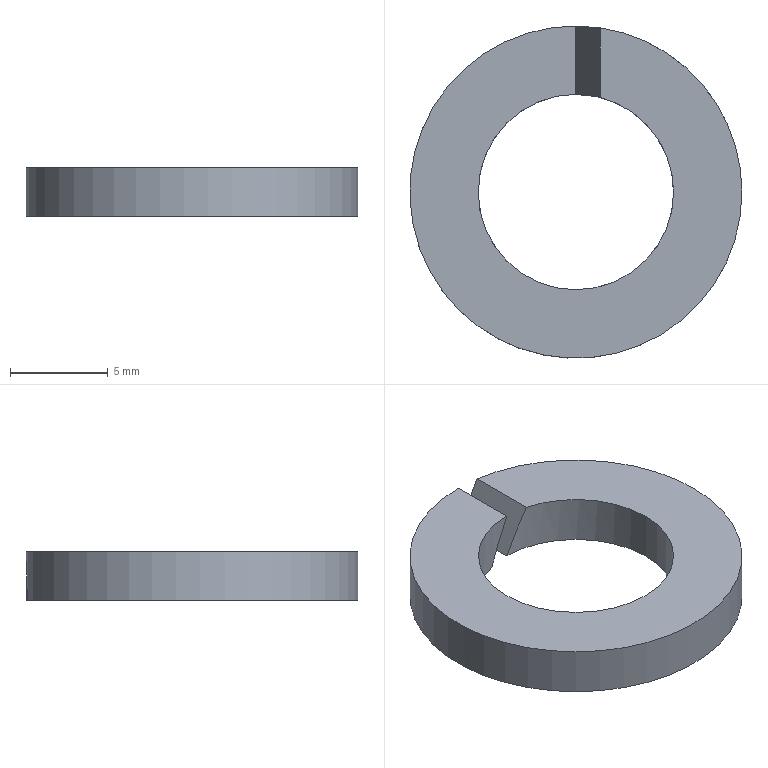Part | STEP file | D10_GB9074_26 | 1 solid | 8 faces | box 17 x 17 x 2.5 mm | volume 360.129 mm3 | plane 4 | cylinder 4 | commonest cylinder face diameters 10 x2 17 x2
STEP:
#1=CARTESIAN_POINT('',(0.,0.,0.));
#2=DIRECTION('',(0.,0.,1.));
#3=DIRECTION('',(1.,0.,0.));
#4=AXIS2_PLACEMENT_3D('',#1,#2,#3);
#5=CARTESIAN_POINT('',(-1.25,4.841,0.));
#6=VERTEX_POINT('',#5);
#7=CARTESIAN_POINT('',(-1.25,8.408,0.));
#8=VERTEX_POINT('',#7);
#9=CARTESIAN_POINT('',(-1.25,4.841,0.));
#10=DIRECTION('',(0.,1.,0.));
#11=VECTOR('',#10,1.);
#12=LINE('',#9,#11);
#13=CARTESIAN_POINT('',(0.,0.,0.));
#14=DIRECTION('',(0.,0.,1.));
#15=DIRECTION('',(1.,0.,0.));
#16=AXIS2_PLACEMENT_3D('',#13,#14,#15);
#17=PLANE('',#16);
#18=CARTESIAN_POINT('',(-1.25,4.841));
#19=DIRECTION('',(0.,1.));
#20=VECTOR('',#19,1.);
#21=LINE('',#18,#20);
#22=(GEOMETRIC_REPRESENTATION_CONTEXT(2)PARAMETRIC_REPRESENTATION_CONTEXT()REPRESENTATION_CONTEXT('',''));
#23=DEFINITIONAL_REPRESENTATION('',(#21),#22);
#24=PCURVE('',#17,#23);
#25=CARTESIAN_POINT('',(-1.25,0.,0.));
#26=DIRECTION('',(-0.8944,0.,0.4472));
#27=DIRECTION('',(0.4472,0.,0.8944));
#28=AXIS2_PLACEMENT_3D('',#25,#26,#27);
#29=PLANE('',#28);
#30=CARTESIAN_POINT('',(0.,4.841));
#31=DIRECTION('',(0.,1.));
#32=VECTOR('',#31,1.);
#33=LINE('',#30,#32);
#34=(GEOMETRIC_REPRESENTATION_CONTEXT(2)PARAMETRIC_REPRESENTATION_CONTEXT()REPRESENTATION_CONTEXT('',''));
#35=DEFINITIONAL_REPRESENTATION('',(#33),#34);
#36=PCURVE('',#29,#35);
#37=SURFACE_CURVE('',#12,(#24,#36),.PCURVE_S1.);
#38=EDGE_CURVE('',#6,#8,#37,.T.);
#39=ORIENTED_EDGE('',*,*,#38,.T.);
#40=CARTESIAN_POINT('',(8.5,0.,0.));
#41=VERTEX_POINT('',#40);
#42=CARTESIAN_POINT('',(0.,0.,0.));
#43=DIRECTION('',(0.,0.,-1.));
#44=DIRECTION('',(1.,0.,0.));
#45=AXIS2_PLACEMENT_3D('',#42,#43,#44);
#46=CIRCLE('',#45,8.5);
#47=CARTESIAN_POINT('',(8.5,0.));
#48=CARTESIAN_POINT('',(8.5,-14.722));
#49=CARTESIAN_POINT('',(-4.25,-7.361));
#50=CARTESIAN_POINT('',(-17.,0.));
#51=CARTESIAN_POINT('',(-4.25,7.361));
#52=CARTESIAN_POINT('',(8.5,14.722));
#53=CARTESIAN_POINT('',(8.5,0.));
#54=(BOUNDED_CURVE()B_SPLINE_CURVE(2,(#47,#48,#49,#50,#51,#52,#53),.UNSPECIFIED.,.T.,.F.)B_SPLINE_CURVE_WITH_KNOTS((1,2,2,2,2,1),(-2.094,0.,2.094,4.189,6.283,8.378),.UNSPECIFIED.)CURVE()GEOMETRIC_REPRESENTATION_ITEM()RATIONAL_B_SPLINE_CURVE((1.,0.5,1.,0.5,1.,0.5,1.))REPRESENTATION_ITEM(''));
#55=(GEOMETRIC_REPRESENTATION_CONTEXT(2)PARAMETRIC_REPRESENTATION_CONTEXT()REPRESENTATION_CONTEXT('',''));
#56=DEFINITIONAL_REPRESENTATION('',(#54),#55);
#57=PCURVE('',#17,#56);
#58=CARTESIAN_POINT('',(0.,0.,0.));
#59=DIRECTION('',(0.,0.,1.));
#60=DIRECTION('',(1.,0.,0.));
#61=AXIS2_PLACEMENT_3D('',#58,#59,#60);
#62=CYLINDRICAL_SURFACE('',#61,8.5);
#63=CARTESIAN_POINT('',(6.283,0.));
#64=DIRECTION('',(-1.,0.));
#65=VECTOR('',#64,1.);
#66=LINE('',#63,#65);
#67=(GEOMETRIC_REPRESENTATION_CONTEXT(2)PARAMETRIC_REPRESENTATION_CONTEXT()REPRESENTATION_CONTEXT('',''));
#68=DEFINITIONAL_REPRESENTATION('',(#66),#67);
#69=PCURVE('',#62,#68);
#70=SURFACE_CURVE('',#46,(#57,#69),.PCURVE_S1.);
#71=EDGE_CURVE('',#41,#8,#70,.T.);
#72=ORIENTED_EDGE('',*,*,#71,.F.);
#73=CARTESIAN_POINT('',(0.,8.5,0.));
#74=VERTEX_POINT('',#73);
#75=CARTESIAN_POINT('',(0.,0.,0.));
#76=DIRECTION('',(0.,0.,1.));
#77=DIRECTION('',(1.,0.,0.));
#78=AXIS2_PLACEMENT_3D('',#75,#76,#77);
#79=CIRCLE('',#78,8.5);
#80=CARTESIAN_POINT('',(0.,0.));
#81=DIRECTION('',(1.,0.));
#82=AXIS2_PLACEMENT_2D('',#80,#81);
#83=CIRCLE('',#82,8.5);
#84=(GEOMETRIC_REPRESENTATION_CONTEXT(2)PARAMETRIC_REPRESENTATION_CONTEXT()REPRESENTATION_CONTEXT('',''));
#85=DEFINITIONAL_REPRESENTATION('',(#83),#84);
#86=PCURVE('',#17,#85);
#87=CARTESIAN_POINT('',(0.,0.,0.));
#88=DIRECTION('',(0.,0.,1.));
#89=DIRECTION('',(1.,0.,0.));
#90=AXIS2_PLACEMENT_3D('',#87,#88,#89);
#91=CYLINDRICAL_SURFACE('',#90,8.5);
#92=CARTESIAN_POINT('',(0.,0.));
#93=DIRECTION('',(1.,0.));
#94=VECTOR('',#93,1.);
#95=LINE('',#92,#94);
#96=(GEOMETRIC_REPRESENTATION_CONTEXT(2)PARAMETRIC_REPRESENTATION_CONTEXT()REPRESENTATION_CONTEXT('',''));
#97=DEFINITIONAL_REPRESENTATION('',(#95),#96);
#98=PCURVE('',#91,#97);
#99=SURFACE_CURVE('',#79,(#86,#98),.PCURVE_S1.);
#100=EDGE_CURVE('',#41,#74,#99,.T.);
#101=ORIENTED_EDGE('',*,*,#100,.T.);
#102=CARTESIAN_POINT('',(0.,5.,0.));
#103=VERTEX_POINT('',#102);
#104=CARTESIAN_POINT('',(0.,5.,0.));
#105=DIRECTION('',(0.,1.,0.));
#106=VECTOR('',#105,1.);
#107=LINE('',#104,#106);
#108=CARTESIAN_POINT('',(0.,5.));
#109=DIRECTION('',(0.,1.));
#110=VECTOR('',#109,1.);
#111=LINE('',#108,#110);
#112=(GEOMETRIC_REPRESENTATION_CONTEXT(2)PARAMETRIC_REPRESENTATION_CONTEXT()REPRESENTATION_CONTEXT('',''));
#113=DEFINITIONAL_REPRESENTATION('',(#111),#112);
#114=PCURVE('',#17,#113);
#115=CARTESIAN_POINT('',(1.25,0.,2.5));
#116=DIRECTION('',(0.8944,0.,-0.4472));
#117=DIRECTION('',(-0.4472,0.,-0.8944));
#118=AXIS2_PLACEMENT_3D('',#115,#116,#117);
#119=PLANE('',#118);
#120=CARTESIAN_POINT('',(2.795,5.));
#121=DIRECTION('',(0.,1.));
#122=VECTOR('',#121,1.);
#123=LINE('',#120,#122);
#124=(GEOMETRIC_REPRESENTATION_CONTEXT(2)PARAMETRIC_REPRESENTATION_CONTEXT()REPRESENTATION_CONTEXT('',''));
#125=DEFINITIONAL_REPRESENTATION('',(#123),#124);
#126=PCURVE('',#119,#125);
#127=SURFACE_CURVE('',#107,(#114,#126),.PCURVE_S1.);
#128=EDGE_CURVE('',#103,#74,#127,.T.);
#129=ORIENTED_EDGE('',*,*,#128,.F.);
#130=CARTESIAN_POINT('',(5.,0.,0.));
#131=VERTEX_POINT('',#130);
#132=CARTESIAN_POINT('',(0.,0.,0.));
#133=DIRECTION('',(0.,0.,-1.));
#134=DIRECTION('',(0.,1.,0.));
#135=AXIS2_PLACEMENT_3D('',#132,#133,#134);
#136=CIRCLE('',#135,5.);
#137=CARTESIAN_POINT('',(0.,5.));
#138=CARTESIAN_POINT('',(8.66,5.));
#139=CARTESIAN_POINT('',(4.33,-2.5));
#140=CARTESIAN_POINT('',(0.,-10.));
#141=CARTESIAN_POINT('',(-4.33,-2.5));
#142=CARTESIAN_POINT('',(-8.66,5.));
#143=CARTESIAN_POINT('',(0.,5.));
#144=(BOUNDED_CURVE()B_SPLINE_CURVE(2,(#137,#138,#139,#140,#141,#142,#143),.UNSPECIFIED.,.T.,.F.)B_SPLINE_CURVE_WITH_KNOTS((1,2,2,2,2,1),(-2.094,0.,2.094,4.189,6.283,8.378),.UNSPECIFIED.)CURVE()GEOMETRIC_REPRESENTATION_ITEM()RATIONAL_B_SPLINE_CURVE((1.,0.5,1.,0.5,1.,0.5,1.))REPRESENTATION_ITEM(''));
#145=(GEOMETRIC_REPRESENTATION_CONTEXT(2)PARAMETRIC_REPRESENTATION_CONTEXT()REPRESENTATION_CONTEXT('',''));
#146=DEFINITIONAL_REPRESENTATION('',(#144),#145);
#147=PCURVE('',#17,#146);
#148=CARTESIAN_POINT('',(0.,0.,0.));
#149=DIRECTION('',(0.,0.,1.));
#150=DIRECTION('',(1.,0.,0.));
#151=AXIS2_PLACEMENT_3D('',#148,#149,#150);
#152=CYLINDRICAL_SURFACE('',#151,5.);
#153=CARTESIAN_POINT('',(1.571,0.));
#154=DIRECTION('',(-1.,0.));
#155=VECTOR('',#154,1.);
#156=LINE('',#153,#155);
#157=(GEOMETRIC_REPRESENTATION_CONTEXT(2)PARAMETRIC_REPRESENTATION_CONTEXT()REPRESENTATION_CONTEXT('',''));
#158=DEFINITIONAL_REPRESENTATION('',(#156),#157);
#159=PCURVE('',#152,#158);
#160=SURFACE_CURVE('',#136,(#147,#159),.PCURVE_S1.);
#161=EDGE_CURVE('',#103,#131,#160,.T.);
#162=ORIENTED_EDGE('',*,*,#161,.T.);
#163=CARTESIAN_POINT('',(0.,0.,0.));
#164=DIRECTION('',(0.,0.,1.));
#165=DIRECTION('',(-0.25,0.9682,0.));
#166=AXIS2_PLACEMENT_3D('',#163,#164,#165);
#167=CIRCLE('',#166,5.);
#168=CARTESIAN_POINT('',(0.,0.));
#169=DIRECTION('',(-0.25,0.9682));
#170=AXIS2_PLACEMENT_2D('',#168,#169);
#171=CIRCLE('',#170,5.);
#172=(GEOMETRIC_REPRESENTATION_CONTEXT(2)PARAMETRIC_REPRESENTATION_CONTEXT()REPRESENTATION_CONTEXT('',''));
#173=DEFINITIONAL_REPRESENTATION('',(#171),#172);
#174=PCURVE('',#17,#173);
#175=CARTESIAN_POINT('',(0.,0.,0.));
#176=DIRECTION('',(0.,0.,1.));
#177=DIRECTION('',(1.,0.,0.));
#178=AXIS2_PLACEMENT_3D('',#175,#176,#177);
#179=CYLINDRICAL_SURFACE('',#178,5.);
#180=CARTESIAN_POINT('',(1.823,0.));
#181=DIRECTION('',(1.,0.));
#182=VECTOR('',#181,1.);
#183=LINE('',#180,#182);
#184=(GEOMETRIC_REPRESENTATION_CONTEXT(2)PARAMETRIC_REPRESENTATION_CONTEXT()REPRESENTATION_CONTEXT('',''));
#185=DEFINITIONAL_REPRESENTATION('',(#183),#184);
#186=PCURVE('',#179,#185);
#187=SURFACE_CURVE('',#167,(#174,#186),.PCURVE_S1.);
#188=EDGE_CURVE('',#6,#131,#187,.T.);
#189=ORIENTED_EDGE('',*,*,#188,.F.);
#190=EDGE_LOOP('',(#39,#72,#101,#129,#162,#189));
#191=FACE_BOUND('',#190,.F.);
#192=ADVANCED_FACE('',(#191),#17,.F.);
#193=CARTESIAN_POINT('',(0.,5.,2.5));
#194=VERTEX_POINT('',#193);
#195=CARTESIAN_POINT('',(0.,5.,2.5));
#196=CARTESIAN_POINT('',(-0.418,5.,1.664));
#197=CARTESIAN_POINT('',(-0.8347,4.948,0.8305));
#198=CARTESIAN_POINT('',(-1.25,4.841,0.));
#199=B_SPLINE_CURVE_WITH_KNOTS('',3,(#195,#196,#197,#198),.UNSPECIFIED.,.F.,.F.,(4,4),(0.,1.),.PIECEWISE_BEZIER_KNOTS.);
#200=CARTESIAN_POINT('',(2.795,5.));
#201=CARTESIAN_POINT('',(1.86,5.));
#202=CARTESIAN_POINT('',(0.9286,4.948));
#203=CARTESIAN_POINT('',(0.,4.841));
#204=B_SPLINE_CURVE_WITH_KNOTS('',3,(#200,#201,#202,#203),.UNSPECIFIED.,.F.,.F.,(4,4),(0.,1.),.PIECEWISE_BEZIER_KNOTS.);
#205=(GEOMETRIC_REPRESENTATION_CONTEXT(2)PARAMETRIC_REPRESENTATION_CONTEXT()REPRESENTATION_CONTEXT('',''));
#206=DEFINITIONAL_REPRESENTATION('',(#204),#205);
#207=PCURVE('',#29,#206);
#208=CARTESIAN_POINT('',(1.571,2.5));
#209=CARTESIAN_POINT('',(1.575,2.462));
#210=CARTESIAN_POINT('',(1.582,2.386));
#211=CARTESIAN_POINT('',(1.594,2.272));
#212=CARTESIAN_POINT('',(1.605,2.158));
#213=CARTESIAN_POINT('',(1.616,2.044));
#214=CARTESIAN_POINT('',(1.628,1.93));
#215=CARTESIAN_POINT('',(1.639,1.817));
#216=CARTESIAN_POINT('',(1.651,1.703));
#217=CARTESIAN_POINT('',(1.662,1.589));
#218=CARTESIAN_POINT('',(1.673,1.475));
#219=CARTESIAN_POINT('',(1.685,1.362));
#220=CARTESIAN_POINT('',(1.696,1.248));
#221=CARTESIAN_POINT('',(1.708,1.134));
#222=CARTESIAN_POINT('',(1.719,1.021));
#223=CARTESIAN_POINT('',(1.731,0.9072));
#224=CARTESIAN_POINT('',(1.742,0.7936));
#225=CARTESIAN_POINT('',(1.754,0.6802));
#226=CARTESIAN_POINT('',(1.765,0.5667));
#227=CARTESIAN_POINT('',(1.777,0.4533));
#228=CARTESIAN_POINT('',(1.789,0.3399));
#229=CARTESIAN_POINT('',(1.8,0.2266));
#230=CARTESIAN_POINT('',(1.812,0.1133));
#231=CARTESIAN_POINT('',(1.82,0.03775));
#232=CARTESIAN_POINT('',(1.823,0.));
#233=B_SPLINE_CURVE_WITH_KNOTS('',3,(#208,#209,#210,#211,#212,#213,#214,#215,#216,#217,#218,#219,#220,#221,#222,#223,#224,#225,#226,#227,#228,#229,#230,#231,#232),.UNSPECIFIED.,.F.,.F.,(4,1,1,1,1,1,1,1,1,1,1,1,1,1,1,1,1,1,1,1,1,1,4),(0.,0.04545,0.09091,0.1364,0.1818,0.2273,0.2727,0.3182,0.3636,0.4091,0.4545,0.5,0.5455,0.5909,0.6364,0.6818,0.7273,0.7727,0.8182,0.8636,0.9091,0.9545,1.),.QUASI_UNIFORM_KNOTS.);
#234=(GEOMETRIC_REPRESENTATION_CONTEXT(2)PARAMETRIC_REPRESENTATION_CONTEXT()REPRESENTATION_CONTEXT('',''));
#235=DEFINITIONAL_REPRESENTATION('',(#233),#234);
#236=PCURVE('',#179,#235);
#237=SURFACE_CURVE('',#199,(#207,#236),.PCURVE_S1.);
#238=EDGE_CURVE('',#194,#6,#237,.T.);
#239=ORIENTED_EDGE('',*,*,#238,.F.);
#240=CARTESIAN_POINT('',(0.,8.5,2.5));
#241=VERTEX_POINT('',#240);
#242=CARTESIAN_POINT('',(0.,5.,2.5));
#243=DIRECTION('',(0.,1.,0.));
#244=VECTOR('',#243,1.);
#245=LINE('',#242,#244);
#246=CARTESIAN_POINT('',(2.795,5.));
#247=DIRECTION('',(0.,1.));
#248=VECTOR('',#247,1.);
#249=LINE('',#246,#248);
#250=(GEOMETRIC_REPRESENTATION_CONTEXT(2)PARAMETRIC_REPRESENTATION_CONTEXT()REPRESENTATION_CONTEXT('',''));
#251=DEFINITIONAL_REPRESENTATION('',(#249),#250);
#252=PCURVE('',#29,#251);
#253=CARTESIAN_POINT('',(0.,0.,2.5));
#254=DIRECTION('',(0.,0.,1.));
#255=DIRECTION('',(1.,0.,0.));
#256=AXIS2_PLACEMENT_3D('',#253,#254,#255);
#257=PLANE('',#256);
#258=CARTESIAN_POINT('',(0.,5.));
#259=DIRECTION('',(0.,1.));
#260=VECTOR('',#259,1.);
#261=LINE('',#258,#260);
#262=(GEOMETRIC_REPRESENTATION_CONTEXT(2)PARAMETRIC_REPRESENTATION_CONTEXT()REPRESENTATION_CONTEXT('',''));
#263=DEFINITIONAL_REPRESENTATION('',(#261),#262);
#264=PCURVE('',#257,#263);
#265=SURFACE_CURVE('',#245,(#252,#264),.PCURVE_S1.);
#266=EDGE_CURVE('',#194,#241,#265,.T.);
#267=ORIENTED_EDGE('',*,*,#266,.T.);
#268=CARTESIAN_POINT('',(0.,8.5,2.5));
#269=CARTESIAN_POINT('',(-0.4171,8.5,1.666));
#270=CARTESIAN_POINT('',(-0.8338,8.469,0.8324));
#271=CARTESIAN_POINT('',(-1.25,8.408,0.));
#272=B_SPLINE_CURVE_WITH_KNOTS('',3,(#268,#269,#270,#271),.UNSPECIFIED.,.F.,.F.,(4,4),(0.,1.),.PIECEWISE_BEZIER_KNOTS.);
#273=CARTESIAN_POINT('',(2.795,8.5));
#274=CARTESIAN_POINT('',(1.862,8.5));
#275=CARTESIAN_POINT('',(0.9307,8.469));
#276=CARTESIAN_POINT('',(0.,8.408));
#277=B_SPLINE_CURVE_WITH_KNOTS('',3,(#273,#274,#275,#276),.UNSPECIFIED.,.F.,.F.,(4,4),(0.,1.),.PIECEWISE_BEZIER_KNOTS.);
#278=(GEOMETRIC_REPRESENTATION_CONTEXT(2)PARAMETRIC_REPRESENTATION_CONTEXT()REPRESENTATION_CONTEXT('',''));
#279=DEFINITIONAL_REPRESENTATION('',(#277),#278);
#280=PCURVE('',#29,#279);
#281=CARTESIAN_POINT('',(1.571,2.5));
#282=CARTESIAN_POINT('',(1.718,0.));
#283=B_SPLINE_CURVE_WITH_KNOTS('',1,(#281,#282),.UNSPECIFIED.,.F.,.F.,(2,2),(0.,1.),.PIECEWISE_BEZIER_KNOTS.);
#284=(GEOMETRIC_REPRESENTATION_CONTEXT(2)PARAMETRIC_REPRESENTATION_CONTEXT()REPRESENTATION_CONTEXT('',''));
#285=DEFINITIONAL_REPRESENTATION('',(#283),#284);
#286=PCURVE('',#62,#285);
#287=SURFACE_CURVE('',#272,(#280,#286),.PCURVE_S1.);
#288=EDGE_CURVE('',#241,#8,#287,.T.);
#289=ORIENTED_EDGE('',*,*,#288,.T.);
#290=ORIENTED_EDGE('',*,*,#38,.F.);
#291=EDGE_LOOP('',(#239,#267,#289,#290));
#292=FACE_BOUND('',#291,.F.);
#293=ADVANCED_FACE('',(#292),#29,.F.);
#294=CARTESIAN_POINT('',(5.,0.,2.5));
#295=VERTEX_POINT('',#294);
#296=CARTESIAN_POINT('',(0.,0.,2.5));
#297=DIRECTION('',(0.,0.,-1.));
#298=DIRECTION('',(1.,0.,0.));
#299=AXIS2_PLACEMENT_3D('',#296,#297,#298);
#300=CIRCLE('',#299,5.);
#301=CARTESIAN_POINT('',(6.283,2.5));
#302=DIRECTION('',(-1.,0.));
#303=VECTOR('',#302,1.);
#304=LINE('',#301,#303);
#305=(GEOMETRIC_REPRESENTATION_CONTEXT(2)PARAMETRIC_REPRESENTATION_CONTEXT()REPRESENTATION_CONTEXT('',''));
#306=DEFINITIONAL_REPRESENTATION('',(#304),#305);
#307=PCURVE('',#179,#306);
#308=CARTESIAN_POINT('',(5.,0.));
#309=CARTESIAN_POINT('',(5.,-8.66));
#310=CARTESIAN_POINT('',(-2.5,-4.33));
#311=CARTESIAN_POINT('',(-10.,0.));
#312=CARTESIAN_POINT('',(-2.5,4.33));
#313=CARTESIAN_POINT('',(5.,8.66));
#314=CARTESIAN_POINT('',(5.,0.));
#315=(BOUNDED_CURVE()B_SPLINE_CURVE(2,(#308,#309,#310,#311,#312,#313,#314),.UNSPECIFIED.,.T.,.F.)B_SPLINE_CURVE_WITH_KNOTS((1,2,2,2,2,1),(-2.094,0.,2.094,4.189,6.283,8.378),.UNSPECIFIED.)CURVE()GEOMETRIC_REPRESENTATION_ITEM()RATIONAL_B_SPLINE_CURVE((1.,0.5,1.,0.5,1.,0.5,1.))REPRESENTATION_ITEM(''));
#316=(GEOMETRIC_REPRESENTATION_CONTEXT(2)PARAMETRIC_REPRESENTATION_CONTEXT()REPRESENTATION_CONTEXT('',''));
#317=DEFINITIONAL_REPRESENTATION('',(#315),#316);
#318=PCURVE('',#257,#317);
#319=SURFACE_CURVE('',#300,(#307,#318),.PCURVE_S1.);
#320=EDGE_CURVE('',#295,#194,#319,.T.);
#321=ORIENTED_EDGE('',*,*,#320,.T.);
#322=ORIENTED_EDGE('',*,*,#238,.T.);
#323=ORIENTED_EDGE('',*,*,#188,.T.);
#324=CARTESIAN_POINT('',(5.,0.,0.));
#325=DIRECTION('',(0.,0.,1.));
#326=VECTOR('',#325,1.);
#327=LINE('',#324,#326);
#328=CARTESIAN_POINT('',(6.283,0.));
#329=DIRECTION('',(0.,1.));
#330=VECTOR('',#329,1.);
#331=LINE('',#328,#330);
#332=(GEOMETRIC_REPRESENTATION_CONTEXT(2)PARAMETRIC_REPRESENTATION_CONTEXT()REPRESENTATION_CONTEXT('',''));
#333=DEFINITIONAL_REPRESENTATION('',(#331),#332);
#334=PCURVE('',#179,#333);
#335=CARTESIAN_POINT('',(0.,0.));
#336=DIRECTION('',(0.,1.));
#337=VECTOR('',#336,1.);
#338=LINE('',#335,#337);
#339=(GEOMETRIC_REPRESENTATION_CONTEXT(2)PARAMETRIC_REPRESENTATION_CONTEXT()REPRESENTATION_CONTEXT('',''));
#340=DEFINITIONAL_REPRESENTATION('',(#338),#339);
#341=PCURVE('',#152,#340);
#342=SURFACE_CURVE('',#327,(#334,#341),.PCURVE_S1.);
#343=EDGE_CURVE('',#131,#295,#342,.T.);
#344=ORIENTED_EDGE('',*,*,#343,.T.);
#345=EDGE_LOOP('',(#321,#322,#323,#344));
#346=FACE_BOUND('',#345,.F.);
#347=ADVANCED_FACE('',(#346),#179,.F.);
#348=ORIENTED_EDGE('',*,*,#266,.F.);
#349=ORIENTED_EDGE('',*,*,#320,.F.);
#350=CARTESIAN_POINT('',(1.25,4.841,2.5));
#351=VERTEX_POINT('',#350);
#352=CARTESIAN_POINT('',(0.,0.,2.5));
#353=DIRECTION('',(0.,0.,-1.));
#354=DIRECTION('',(0.25,0.9682,0.));
#355=AXIS2_PLACEMENT_3D('',#352,#353,#354);
#356=CIRCLE('',#355,5.);
#357=CARTESIAN_POINT('',(1.25,4.841));
#358=CARTESIAN_POINT('',(9.635,2.676));
#359=CARTESIAN_POINT('',(3.568,-3.503));
#360=CARTESIAN_POINT('',(-2.5,-9.682));
#361=CARTESIAN_POINT('',(-4.818,-1.338));
#362=CARTESIAN_POINT('',(-7.135,7.006));
#363=CARTESIAN_POINT('',(1.25,4.841));
#364=(BOUNDED_CURVE()B_SPLINE_CURVE(2,(#357,#358,#359,#360,#361,#362,#363),.UNSPECIFIED.,.T.,.F.)B_SPLINE_CURVE_WITH_KNOTS((1,2,2,2,2,1),(-2.094,0.,2.094,4.189,6.283,8.378),.UNSPECIFIED.)CURVE()GEOMETRIC_REPRESENTATION_ITEM()RATIONAL_B_SPLINE_CURVE((1.,0.5,1.,0.5,1.,0.5,1.))REPRESENTATION_ITEM(''));
#365=(GEOMETRIC_REPRESENTATION_CONTEXT(2)PARAMETRIC_REPRESENTATION_CONTEXT()REPRESENTATION_CONTEXT('',''));
#366=DEFINITIONAL_REPRESENTATION('',(#364),#365);
#367=PCURVE('',#257,#366);
#368=CARTESIAN_POINT('',(1.318,2.5));
#369=DIRECTION('',(-1.,0.));
#370=VECTOR('',#369,1.);
#371=LINE('',#368,#370);
#372=(GEOMETRIC_REPRESENTATION_CONTEXT(2)PARAMETRIC_REPRESENTATION_CONTEXT()REPRESENTATION_CONTEXT('',''));
#373=DEFINITIONAL_REPRESENTATION('',(#371),#372);
#374=PCURVE('',#152,#373);
#375=SURFACE_CURVE('',#356,(#367,#374),.PCURVE_S1.);
#376=EDGE_CURVE('',#351,#295,#375,.T.);
#377=ORIENTED_EDGE('',*,*,#376,.F.);
#378=CARTESIAN_POINT('',(1.25,8.408,2.5));
#379=VERTEX_POINT('',#378);
#380=CARTESIAN_POINT('',(1.25,4.841,2.5));
#381=DIRECTION('',(0.,1.,0.));
#382=VECTOR('',#381,1.);
#383=LINE('',#380,#382);
#384=CARTESIAN_POINT('',(1.25,4.841));
#385=DIRECTION('',(0.,1.));
#386=VECTOR('',#385,1.);
#387=LINE('',#384,#386);
#388=(GEOMETRIC_REPRESENTATION_CONTEXT(2)PARAMETRIC_REPRESENTATION_CONTEXT()REPRESENTATION_CONTEXT('',''));
#389=DEFINITIONAL_REPRESENTATION('',(#387),#388);
#390=PCURVE('',#257,#389);
#391=CARTESIAN_POINT('',(0.,4.841));
#392=DIRECTION('',(0.,1.));
#393=VECTOR('',#392,1.);
#394=LINE('',#391,#393);
#395=(GEOMETRIC_REPRESENTATION_CONTEXT(2)PARAMETRIC_REPRESENTATION_CONTEXT()REPRESENTATION_CONTEXT('',''));
#396=DEFINITIONAL_REPRESENTATION('',(#394),#395);
#397=PCURVE('',#119,#396);
#398=SURFACE_CURVE('',#383,(#390,#397),.PCURVE_S1.);
#399=EDGE_CURVE('',#351,#379,#398,.T.);
#400=ORIENTED_EDGE('',*,*,#399,.T.);
#401=CARTESIAN_POINT('',(8.5,0.,2.5));
#402=VERTEX_POINT('',#401);
#403=CARTESIAN_POINT('',(0.,0.,2.5));
#404=DIRECTION('',(0.,0.,1.));
#405=DIRECTION('',(1.,0.,0.));
#406=AXIS2_PLACEMENT_3D('',#403,#404,#405);
#407=CIRCLE('',#406,8.5);
#408=CARTESIAN_POINT('',(0.,0.));
#409=DIRECTION('',(1.,0.));
#410=AXIS2_PLACEMENT_2D('',#408,#409);
#411=CIRCLE('',#410,8.5);
#412=(GEOMETRIC_REPRESENTATION_CONTEXT(2)PARAMETRIC_REPRESENTATION_CONTEXT()REPRESENTATION_CONTEXT('',''));
#413=DEFINITIONAL_REPRESENTATION('',(#411),#412);
#414=PCURVE('',#257,#413);
#415=CARTESIAN_POINT('',(0.,2.5));
#416=DIRECTION('',(1.,0.));
#417=VECTOR('',#416,1.);
#418=LINE('',#415,#417);
#419=(GEOMETRIC_REPRESENTATION_CONTEXT(2)PARAMETRIC_REPRESENTATION_CONTEXT()REPRESENTATION_CONTEXT('',''));
#420=DEFINITIONAL_REPRESENTATION('',(#418),#419);
#421=PCURVE('',#91,#420);
#422=SURFACE_CURVE('',#407,(#414,#421),.PCURVE_S1.);
#423=EDGE_CURVE('',#402,#379,#422,.T.);
#424=ORIENTED_EDGE('',*,*,#423,.F.);
#425=CARTESIAN_POINT('',(0.,0.,2.5));
#426=DIRECTION('',(0.,0.,1.));
#427=DIRECTION('',(0.,1.,0.));
#428=AXIS2_PLACEMENT_3D('',#425,#426,#427);
#429=CIRCLE('',#428,8.5);
#430=CARTESIAN_POINT('',(0.,0.));
#431=DIRECTION('',(0.,1.));
#432=AXIS2_PLACEMENT_2D('',#430,#431);
#433=CIRCLE('',#432,8.5);
#434=(GEOMETRIC_REPRESENTATION_CONTEXT(2)PARAMETRIC_REPRESENTATION_CONTEXT()REPRESENTATION_CONTEXT('',''));
#435=DEFINITIONAL_REPRESENTATION('',(#433),#434);
#436=PCURVE('',#257,#435);
#437=CARTESIAN_POINT('',(1.571,2.5));
#438=DIRECTION('',(1.,0.));
#439=VECTOR('',#438,1.);
#440=LINE('',#437,#439);
#441=(GEOMETRIC_REPRESENTATION_CONTEXT(2)PARAMETRIC_REPRESENTATION_CONTEXT()REPRESENTATION_CONTEXT('',''));
#442=DEFINITIONAL_REPRESENTATION('',(#440),#441);
#443=PCURVE('',#62,#442);
#444=SURFACE_CURVE('',#429,(#436,#443),.PCURVE_S1.);
#445=EDGE_CURVE('',#241,#402,#444,.T.);
#446=ORIENTED_EDGE('',*,*,#445,.F.);
#447=EDGE_LOOP('',(#348,#349,#377,#400,#424,#446));
#448=FACE_BOUND('',#447,.F.);
#449=ADVANCED_FACE('',(#448),#257,.T.);
#450=CARTESIAN_POINT('',(1.25,4.841,2.5));
#451=CARTESIAN_POINT('',(0.8347,4.948,1.669));
#452=CARTESIAN_POINT('',(0.418,5.,0.8361));
#453=CARTESIAN_POINT('',(0.,5.,0.));
#454=B_SPLINE_CURVE_WITH_KNOTS('',3,(#450,#451,#452,#453),.UNSPECIFIED.,.F.,.F.,(4,4),(0.,1.),.PIECEWISE_BEZIER_KNOTS.);
#455=CARTESIAN_POINT('',(1.318,2.5));
#456=CARTESIAN_POINT('',(1.322,2.462));
#457=CARTESIAN_POINT('',(1.33,2.387));
#458=CARTESIAN_POINT('',(1.341,2.273));
#459=CARTESIAN_POINT('',(1.353,2.16));
#460=CARTESIAN_POINT('',(1.365,2.047));
#461=CARTESIAN_POINT('',(1.376,1.933));
#462=CARTESIAN_POINT('',(1.388,1.82));
#463=CARTESIAN_POINT('',(1.399,1.706));
#464=CARTESIAN_POINT('',(1.411,1.593));
#465=CARTESIAN_POINT('',(1.422,1.479));
#466=CARTESIAN_POINT('',(1.434,1.366));
#467=CARTESIAN_POINT('',(1.445,1.252));
#468=CARTESIAN_POINT('',(1.457,1.138));
#469=CARTESIAN_POINT('',(1.468,1.025));
#470=CARTESIAN_POINT('',(1.48,0.911));
#471=CARTESIAN_POINT('',(1.491,0.7972));
#472=CARTESIAN_POINT('',(1.502,0.6835));
#473=CARTESIAN_POINT('',(1.514,0.5696));
#474=CARTESIAN_POINT('',(1.525,0.4558));
#475=CARTESIAN_POINT('',(1.537,0.3419));
#476=CARTESIAN_POINT('',(1.548,0.228));
#477=CARTESIAN_POINT('',(1.559,0.114));
#478=CARTESIAN_POINT('',(1.567,0.038));
#479=CARTESIAN_POINT('',(1.571,0.));
#480=B_SPLINE_CURVE_WITH_KNOTS('',3,(#455,#456,#457,#458,#459,#460,#461,#462,#463,#464,#465,#466,#467,#468,#469,#470,#471,#472,#473,#474,#475,#476,#477,#478,#479),.UNSPECIFIED.,.F.,.F.,(4,1,1,1,1,1,1,1,1,1,1,1,1,1,1,1,1,1,1,1,1,1,4),(0.,0.04545,0.09091,0.1364,0.1818,0.2273,0.2727,0.3182,0.3636,0.4091,0.4545,0.5,0.5455,0.5909,0.6364,0.6818,0.7273,0.7727,0.8182,0.8636,0.9091,0.9545,1.),.QUASI_UNIFORM_KNOTS.);
#481=(GEOMETRIC_REPRESENTATION_CONTEXT(2)PARAMETRIC_REPRESENTATION_CONTEXT()REPRESENTATION_CONTEXT('',''));
#482=DEFINITIONAL_REPRESENTATION('',(#480),#481);
#483=PCURVE('',#152,#482);
#484=CARTESIAN_POINT('',(0.,4.841));
#485=CARTESIAN_POINT('',(0.9286,4.948));
#486=CARTESIAN_POINT('',(1.86,5.));
#487=CARTESIAN_POINT('',(2.795,5.));
#488=B_SPLINE_CURVE_WITH_KNOTS('',3,(#484,#485,#486,#487),.UNSPECIFIED.,.F.,.F.,(4,4),(0.,1.),.PIECEWISE_BEZIER_KNOTS.);
#489=(GEOMETRIC_REPRESENTATION_CONTEXT(2)PARAMETRIC_REPRESENTATION_CONTEXT()REPRESENTATION_CONTEXT('',''));
#490=DEFINITIONAL_REPRESENTATION('',(#488),#489);
#491=PCURVE('',#119,#490);
#492=SURFACE_CURVE('',#454,(#483,#491),.PCURVE_S1.);
#493=EDGE_CURVE('',#351,#103,#492,.T.);
#494=ORIENTED_EDGE('',*,*,#493,.F.);
#495=ORIENTED_EDGE('',*,*,#376,.T.);
#496=ORIENTED_EDGE('',*,*,#343,.F.);
#497=ORIENTED_EDGE('',*,*,#161,.F.);
#498=EDGE_LOOP('',(#494,#495,#496,#497));
#499=FACE_BOUND('',#498,.F.);
#500=ADVANCED_FACE('',(#499),#152,.F.);
#501=CARTESIAN_POINT('',(1.25,8.408,2.5));
#502=CARTESIAN_POINT('',(0.8338,8.469,1.668));
#503=CARTESIAN_POINT('',(0.4171,8.5,0.8342));
#504=CARTESIAN_POINT('',(0.,8.5,0.));
#505=B_SPLINE_CURVE_WITH_KNOTS('',3,(#501,#502,#503,#504),.UNSPECIFIED.,.F.,.F.,(4,4),(0.,1.),.PIECEWISE_BEZIER_KNOTS.);
#506=CARTESIAN_POINT('',(0.,8.408));
#507=CARTESIAN_POINT('',(0.9307,8.469));
#508=CARTESIAN_POINT('',(1.862,8.5));
#509=CARTESIAN_POINT('',(2.795,8.5));
#510=B_SPLINE_CURVE_WITH_KNOTS('',3,(#506,#507,#508,#509),.UNSPECIFIED.,.F.,.F.,(4,4),(0.,1.),.PIECEWISE_BEZIER_KNOTS.);
#511=(GEOMETRIC_REPRESENTATION_CONTEXT(2)PARAMETRIC_REPRESENTATION_CONTEXT()REPRESENTATION_CONTEXT('',''));
#512=DEFINITIONAL_REPRESENTATION('',(#510),#511);
#513=PCURVE('',#119,#512);
#514=CARTESIAN_POINT('',(1.423,2.5));
#515=CARTESIAN_POINT('',(1.571,0.));
#516=B_SPLINE_CURVE_WITH_KNOTS('',1,(#514,#515),.UNSPECIFIED.,.F.,.F.,(2,2),(0.,1.),.PIECEWISE_BEZIER_KNOTS.);
#517=(GEOMETRIC_REPRESENTATION_CONTEXT(2)PARAMETRIC_REPRESENTATION_CONTEXT()REPRESENTATION_CONTEXT('',''));
#518=DEFINITIONAL_REPRESENTATION('',(#516),#517);
#519=PCURVE('',#91,#518);
#520=SURFACE_CURVE('',#505,(#513,#519),.PCURVE_S1.);
#521=EDGE_CURVE('',#379,#74,#520,.T.);
#522=ORIENTED_EDGE('',*,*,#521,.F.);
#523=ORIENTED_EDGE('',*,*,#399,.F.);
#524=ORIENTED_EDGE('',*,*,#493,.T.);
#525=ORIENTED_EDGE('',*,*,#128,.T.);
#526=EDGE_LOOP('',(#522,#523,#524,#525));
#527=FACE_BOUND('',#526,.F.);
#528=ADVANCED_FACE('',(#527),#119,.F.);
#529=ORIENTED_EDGE('',*,*,#423,.F.);
#530=CARTESIAN_POINT('',(8.5,0.,0.));
#531=DIRECTION('',(0.,0.,1.));
#532=VECTOR('',#531,1.);
#533=LINE('',#530,#532);
#534=CARTESIAN_POINT('',(0.,0.));
#535=DIRECTION('',(0.,1.));
#536=VECTOR('',#535,1.);
#537=LINE('',#534,#536);
#538=(GEOMETRIC_REPRESENTATION_CONTEXT(2)PARAMETRIC_REPRESENTATION_CONTEXT()REPRESENTATION_CONTEXT('',''));
#539=DEFINITIONAL_REPRESENTATION('',(#537),#538);
#540=PCURVE('',#91,#539);
#541=CARTESIAN_POINT('',(6.283,0.));
#542=DIRECTION('',(0.,1.));
#543=VECTOR('',#542,1.);
#544=LINE('',#541,#543);
#545=(GEOMETRIC_REPRESENTATION_CONTEXT(2)PARAMETRIC_REPRESENTATION_CONTEXT()REPRESENTATION_CONTEXT('',''));
#546=DEFINITIONAL_REPRESENTATION('',(#544),#545);
#547=PCURVE('',#62,#546);
#548=SURFACE_CURVE('',#533,(#540,#547),.PCURVE_S1.);
#549=EDGE_CURVE('',#41,#402,#548,.T.);
#550=ORIENTED_EDGE('',*,*,#549,.F.);
#551=ORIENTED_EDGE('',*,*,#100,.T.);
#552=ORIENTED_EDGE('',*,*,#521,.F.);
#553=EDGE_LOOP('',(#529,#550,#551,#552));
#554=FACE_BOUND('',#553,.T.);
#555=ADVANCED_FACE('',(#554),#91,.T.);
#556=ORIENTED_EDGE('',*,*,#549,.T.);
#557=ORIENTED_EDGE('',*,*,#445,.F.);
#558=ORIENTED_EDGE('',*,*,#288,.T.);
#559=ORIENTED_EDGE('',*,*,#71,.F.);
#560=EDGE_LOOP('',(#556,#557,#558,#559));
#561=FACE_BOUND('',#560,.T.);
#562=ADVANCED_FACE('',(#561),#62,.T.);
#563=CLOSED_SHELL('',(#192,#293,#347,#449,#500,#528,#555,#562));
#564=MANIFOLD_SOLID_BREP('',#563);
#565=(LENGTH_UNIT()NAMED_UNIT(*)SI_UNIT(.MILLI.,.METRE.));
#566=UNCERTAINTY_MEASURE_WITH_UNIT(LENGTH_MEASURE(0.0005),#565,'','');
#567=(NAMED_UNIT(*)PLANE_ANGLE_UNIT()SI_UNIT($,.RADIAN.));
#568=(NAMED_UNIT(*)SI_UNIT($,.STERADIAN.)SOLID_ANGLE_UNIT());
#569=(GEOMETRIC_REPRESENTATION_CONTEXT(3)GLOBAL_UNCERTAINTY_ASSIGNED_CONTEXT((#566))GLOBAL_UNIT_ASSIGNED_CONTEXT((#565,#567,#568))REPRESENTATION_CONTEXT('',''));
#570=ADVANCED_BREP_SHAPE_REPRESENTATION('',(#4,#564),#569);